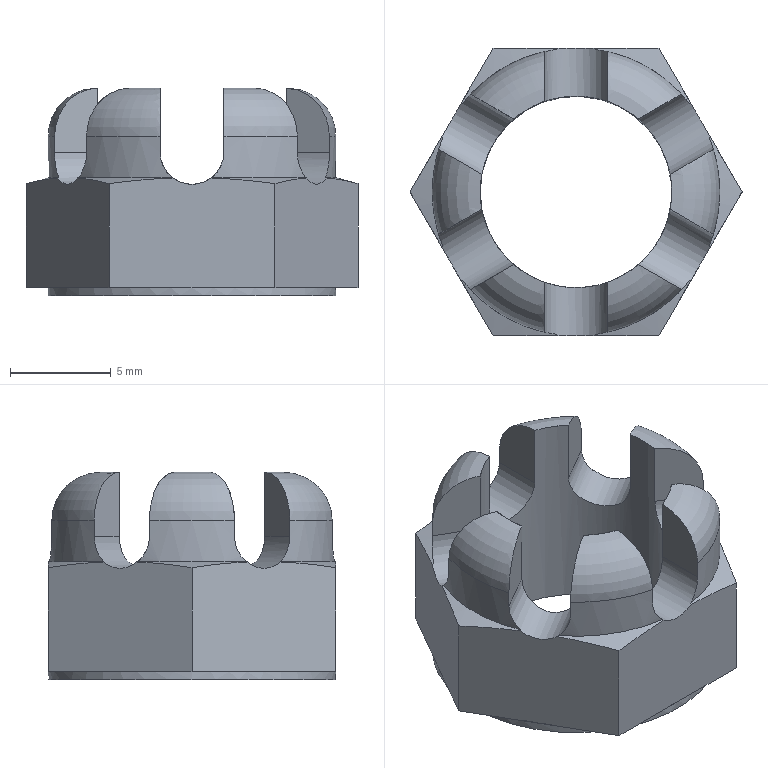Part | NX | features solid 2 | 1 solid | 57 faces | box 16.512 x 14.3 x 10.319 mm | volume 778.974 mm3 | plane 31 | cylinder 14 | torus 6 | cone 6 | commonest cylinder face diameters 14.3 x7 3.175 x6 9.525 x1